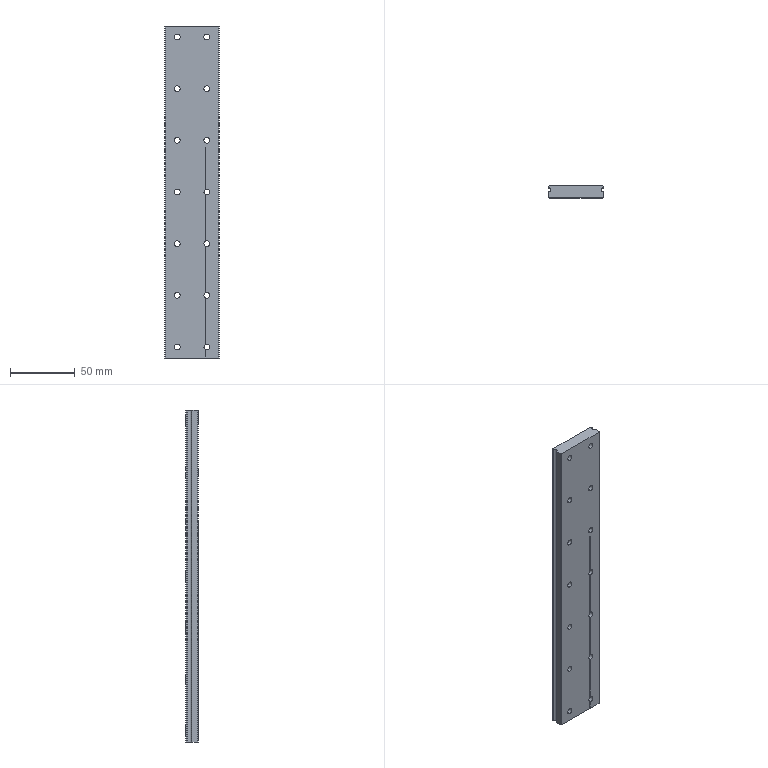Part | STEP file | Bag feed MGW15H slide rail | 1 solid | 91 faces | box 42 x 9.5 x 257 mm | volume 96343 mm3 | cylinder 64 | plane 27 | commonest cylinder face diameters 4.5 x28 8 x28 0.6 x5 3 x3